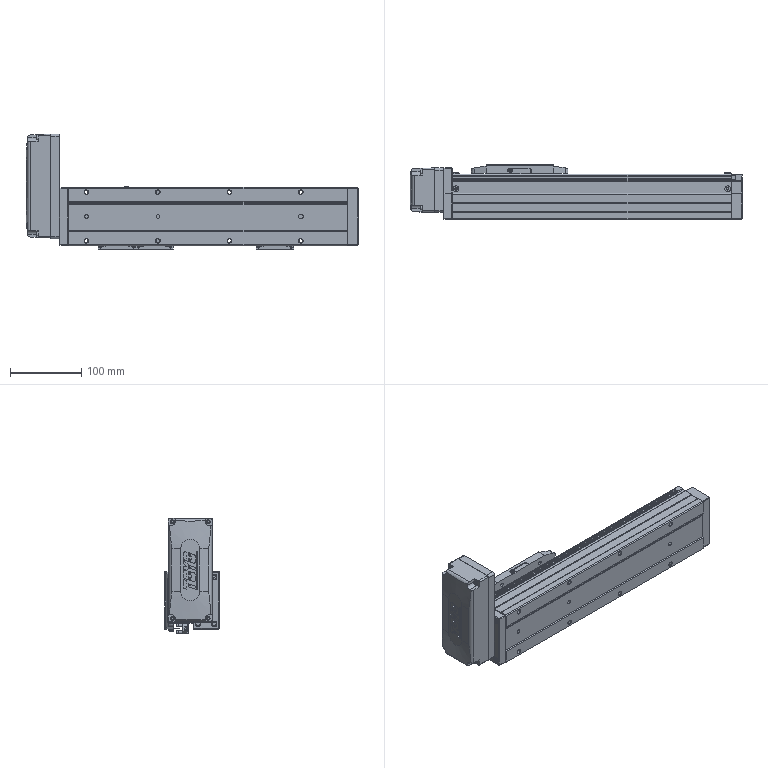Part | SolidWorks | features BaseBody 14 | 14 solids | 1502 faces | box 464.5 x 78 x 161.5 mm | volume 2357243 mm3 | plane 957 | cylinder 407 | cone 78 | torus 60 | commonest cylinder face diameters 1 x40 5.5 x40 2 x36 8 x32 7 x28 4 x27